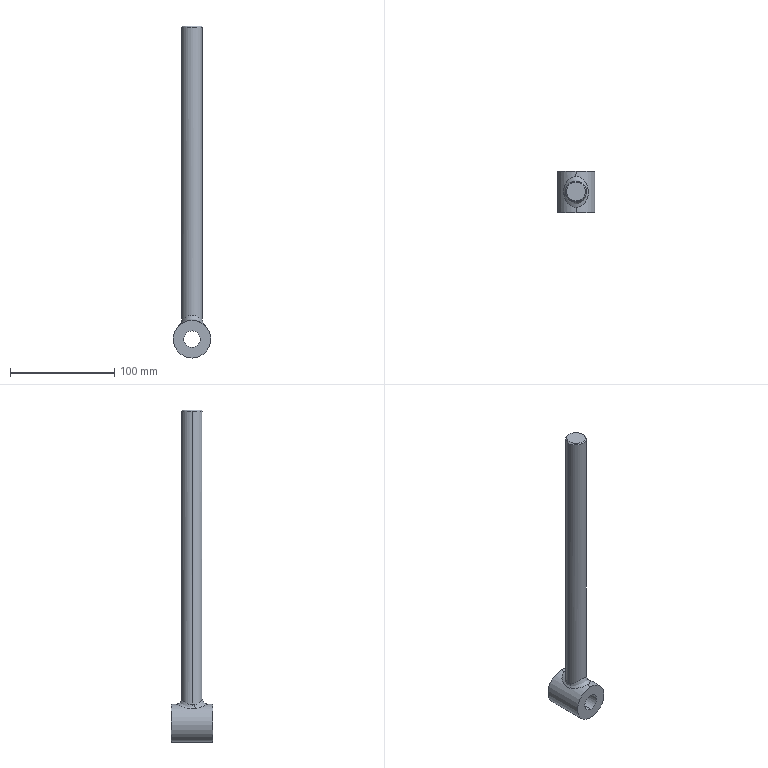Part | SolidWorks | 1 solid | 13 faces | box 36 x 40 x 318 mm | volume 121648 mm3 | cylinder 6 | plane 3 | cone 2 | spline 2 | commonest cylinder face diameters 16 x2 20 x2 36 x2
STEP:
#1=CARTESIAN_POINT('',(9.,0.,300.));
#2=VERTEX_POINT('',#1);
#3=CARTESIAN_POINT('',(-9.,0.,300.));
#4=VERTEX_POINT('',#3);
#5=CARTESIAN_POINT('',(0.,0.,300.));
#6=DIRECTION('',(0.,0.,1.));
#7=DIRECTION('',(1.,0.,0.));
#8=AXIS2_PLACEMENT_3D('',#5,#6,#7);
#9=CIRCLE('',#8,9.);
#10=EDGE_CURVE('',#2,#4,#9,.T.);
#11=ORIENTED_EDGE('',*,*,#10,.F.);
#12=CARTESIAN_POINT('',(10.,0.,299.));
#13=VERTEX_POINT('',#12);
#14=CARTESIAN_POINT('',(9.,0.,300.));
#15=DIRECTION('',(0.7071,0.,-0.7071));
#16=VECTOR('',#15,1000.);
#17=LINE('',#14,#16);
#18=EDGE_CURVE('',#2,#13,#17,.T.);
#19=ORIENTED_EDGE('',*,*,#18,.T.);
#20=CARTESIAN_POINT('',(-10.,0.,299.));
#21=VERTEX_POINT('',#20);
#22=CARTESIAN_POINT('',(0.,0.,299.));
#23=DIRECTION('',(0.,0.,-1.));
#24=DIRECTION('',(1.,0.,0.));
#25=AXIS2_PLACEMENT_3D('',#22,#23,#24);
#26=CIRCLE('',#25,10.);
#27=EDGE_CURVE('',#21,#13,#26,.T.);
#28=ORIENTED_EDGE('',*,*,#27,.F.);
#29=CARTESIAN_POINT('',(-9.,0.,300.));
#30=DIRECTION('',(-0.7071,0.,-0.7071));
#31=VECTOR('',#30,1000.);
#32=LINE('',#29,#31);
#33=EDGE_CURVE('',#4,#21,#32,.T.);
#34=ORIENTED_EDGE('',*,*,#33,.F.);
#35=EDGE_LOOP('',(#11,#19,#28,#34));
#36=FACE_OUTER_BOUND('',#35,.T.);
#37=CARTESIAN_POINT('',(0.,0.,300.));
#38=DIRECTION('',(0.,0.,-1.));
#39=DIRECTION('',(-1.,0.,0.));
#40=AXIS2_PLACEMENT_3D('',#37,#38,#39);
#41=CONICAL_SURFACE('',#40,9.,0.7854);
#42=ADVANCED_FACE('',(#36),#41,.T.);
#43=CARTESIAN_POINT('',(11.46,3.254,13.881));
#44=VERTEX_POINT('',#43);
#45=CARTESIAN_POINT('',(0.,-15.,18.));
#46=VERTEX_POINT('',#45);
#47=CARTESIAN_POINT('',(11.46,3.254,13.881));
#48=CARTESIAN_POINT('',(11.548,2.746,13.808));
#49=CARTESIAN_POINT('',(11.615,2.233,13.751));
#50=CARTESIAN_POINT('',(11.709,1.199,13.672));
#51=CARTESIAN_POINT('',(11.734,0.6762,13.649));
#52=CARTESIAN_POINT('',(11.747,-0.8792,13.638));
#53=CARTESIAN_POINT('',(11.672,-1.908,13.704));
#54=CARTESIAN_POINT('',(11.433,-3.441,13.903));
#55=CARTESIAN_POINT('',(11.333,-3.946,13.985));
#56=CARTESIAN_POINT('',(11.093,-4.936,14.176));
#57=CARTESIAN_POINT('',(10.953,-5.422,14.285));
#58=CARTESIAN_POINT('',(10.632,-6.379,14.526));
#59=CARTESIAN_POINT('',(10.451,-6.851,14.657));
#60=CARTESIAN_POINT('',(10.05,-7.77,14.935));
#61=CARTESIAN_POINT('',(9.83,-8.216,15.081));
#62=CARTESIAN_POINT('',(9.351,-9.083,15.383));
#63=CARTESIAN_POINT('',(9.092,-9.504,15.538));
#64=CARTESIAN_POINT('',(8.531,-10.319,15.853));
#65=CARTESIAN_POINT('',(8.227,-10.715,16.014));
#66=CARTESIAN_POINT('',(7.262,-11.838,16.486));
#67=CARTESIAN_POINT('',(6.545,-12.509,16.79));
#68=CARTESIAN_POINT('',(5.326,-13.38,17.199));
#69=CARTESIAN_POINT('',(4.892,-13.65,17.329));
#70=CARTESIAN_POINT('',(3.994,-14.119,17.557));
#71=CARTESIAN_POINT('',(3.529,-14.32,17.657));
#72=CARTESIAN_POINT('',(2.807,-14.568,17.781));
#73=CARTESIAN_POINT('',(2.562,-14.642,17.819));
#74=CARTESIAN_POINT('',(2.063,-14.77,17.883));
#75=CARTESIAN_POINT('',(1.808,-14.825,17.911));
#76=CARTESIAN_POINT('',(1.035,-14.956,17.978));
#77=CARTESIAN_POINT('',(0.518,-15.,18.));
#78=CARTESIAN_POINT('',(0.,-15.,18.));
#79=B_SPLINE_CURVE_WITH_KNOTS('',3,(#47,#48,#49,#50,#51,#52,#53,#54,#55,#56,#57,#58,#59,#60,#61,#62,#63,#64,#65,#66,#67,#68,#69,#70,#71,#72,#73,#74,#75,#76,#77,#78),.UNSPECIFIED.,.F.,.F.,(4,2,2,2,2,2,2,2,2,2,2,2,2,2,2,4),(0.04024,0.04181,0.04337,0.04651,0.04808,0.04964,0.05121,0.05278,0.05435,0.05592,0.05905,0.06062,0.06219,0.06297,0.06375,0.06532),.UNSPECIFIED.);
#80=EDGE_CURVE('',#44,#46,#79,.T.);
#81=ORIENTED_EDGE('',*,*,#80,.F.);
#82=CARTESIAN_POINT('',(9.762,2.169,17.737));
#83=VERTEX_POINT('',#82);
#84=CARTESIAN_POINT('',(14.643,3.254,17.737));
#85=DIRECTION('',(-0.2135,0.9609,0.1763));
#86=DIRECTION('',(-0.9762,-0.2169,0.));
#87=AXIS2_PLACEMENT_3D('',#84,#85,#86);
#88=CIRCLE('',#87,5.);
#89=EDGE_CURVE('',#44,#83,#88,.T.);
#90=ORIENTED_EDGE('',*,*,#89,.T.);
#91=CARTESIAN_POINT('',(10.,0.,17.436));
#92=VERTEX_POINT('',#91);
#93=CARTESIAN_POINT('',(10.,0.,17.436));
#94=CARTESIAN_POINT('',(10.,0.3703,17.436));
#95=CARTESIAN_POINT('',(9.979,0.7418,17.463));
#96=CARTESIAN_POINT('',(9.899,1.467,17.566));
#97=CARTESIAN_POINT('',(9.839,1.822,17.641));
#98=CARTESIAN_POINT('',(9.762,2.169,17.737));
#99=B_SPLINE_CURVE_WITH_KNOTS('',3,(#93,#94,#95,#96,#97,#98),.UNSPECIFIED.,.F.,.F.,(4,2,4),(0.03372,0.03482,0.03592),.UNSPECIFIED.);
#100=EDGE_CURVE('',#92,#83,#99,.T.);
#101=ORIENTED_EDGE('',*,*,#100,.F.);
#102=CARTESIAN_POINT('',(-9.771,-2.127,17.725));
#103=VERTEX_POINT('',#102);
#104=CARTESIAN_POINT('',(-9.771,-2.127,17.725));
#105=CARTESIAN_POINT('',(-9.634,-2.757,17.895));
#106=CARTESIAN_POINT('',(-9.445,-3.34,18.124));
#107=CARTESIAN_POINT('',(-9.096,-4.166,18.517));
#108=CARTESIAN_POINT('',(-8.968,-4.433,18.657));
#109=CARTESIAN_POINT('',(-8.692,-4.954,18.949));
#110=CARTESIAN_POINT('',(-8.542,-5.207,19.102));
#111=CARTESIAN_POINT('',(-8.066,-5.939,19.568));
#112=CARTESIAN_POINT('',(-7.714,-6.39,19.889));
#113=CARTESIAN_POINT('',(-6.931,-7.231,20.527));
#114=CARTESIAN_POINT('',(-6.499,-7.623,20.846));
#115=CARTESIAN_POINT('',(-5.565,-8.329,21.445));
#116=CARTESIAN_POINT('',(-5.064,-8.645,21.726));
#117=CARTESIAN_POINT('',(-4.247,-9.058,22.104));
#118=CARTESIAN_POINT('',(-3.964,-9.186,22.223));
#119=CARTESIAN_POINT('',(-3.386,-9.414,22.437));
#120=CARTESIAN_POINT('',(-3.09,-9.516,22.533));
#121=CARTESIAN_POINT('',(-2.483,-9.692,22.701));
#122=CARTESIAN_POINT('',(-2.172,-9.767,22.773));
#123=CARTESIAN_POINT('',(-1.532,-9.887,22.89));
#124=CARTESIAN_POINT('',(-1.205,-9.933,22.934));
#125=CARTESIAN_POINT('',(-0.5528,-9.99,22.99));
#126=CARTESIAN_POINT('',(-0.2258,-10.003,23.003));
#127=CARTESIAN_POINT('',(0.4303,-9.996,22.996));
#128=CARTESIAN_POINT('',(0.7605,-9.977,22.977));
#129=CARTESIAN_POINT('',(1.418,-9.905,22.907));
#130=CARTESIAN_POINT('',(1.743,-9.852,22.856));
#131=CARTESIAN_POINT('',(2.373,-9.72,22.728));
#132=CARTESIAN_POINT('',(2.68,-9.639,22.651));
#133=CARTESIAN_POINT('',(3.28,-9.452,22.472));
#134=CARTESIAN_POINT('',(3.572,-9.345,22.372));
#135=CARTESIAN_POINT('',(4.144,-9.106,22.149));
#136=CARTESIAN_POINT('',(4.423,-8.974,22.026));
#137=CARTESIAN_POINT('',(5.225,-8.548,21.64));
#138=CARTESIAN_POINT('',(5.716,-8.226,21.355));
#139=CARTESIAN_POINT('',(6.4,-7.689,20.904));
#140=CARTESIAN_POINT('',(6.619,-7.502,20.75));
#141=CARTESIAN_POINT('',(7.04,-7.108,20.435));
#142=CARTESIAN_POINT('',(7.243,-6.9,20.275));
#143=CARTESIAN_POINT('',(7.82,-6.259,19.795));
#144=CARTESIAN_POINT('',(8.166,-5.802,19.475));
#145=CARTESIAN_POINT('',(8.782,-4.818,18.862));
#146=CARTESIAN_POINT('',(9.055,-4.287,18.566));
#147=CARTESIAN_POINT('',(9.392,-3.448,18.182));
#148=CARTESIAN_POINT('',(9.493,-3.16,18.063));
#149=CARTESIAN_POINT('',(9.67,-2.566,17.85));
#150=CARTESIAN_POINT('',(9.747,-2.258,17.755));
#151=CARTESIAN_POINT('',(9.935,-1.311,17.521));
#152=CARTESIAN_POINT('',(10.,-0.6645,17.436));
#153=CARTESIAN_POINT('',(10.,0.,17.436));
#154=B_SPLINE_CURVE_WITH_KNOTS('',3,(#104,#105,#106,#107,#108,#109,#110,#111,#112,#113,#114,#115,#116,#117,#118,#119,#120,#121,#122,#123,#124,#125,#126,#127,#128,#129,#130,#131,#132,#133,#134,#135,#136,#137,#138,#139,#140,#141,#142,#143,#144,#145,#146,#147,#148,#149,#150,#151,#152,#153),.UNSPECIFIED.,.F.,.F.,(4,2,2,2,2,2,2,2,2,2,2,2,2,2,2,2,2,2,2,2,2,2,2,2,4),(0.002159,0.004132,0.005118,0.006104,0.008077,0.01005,0.01202,0.01301,0.01399,0.01498,0.01597,0.01695,0.01794,0.01893,0.01991,0.0209,0.02189,0.02386,0.02484,0.02583,0.0278,0.02978,0.03076,0.03175,0.03372),.UNSPECIFIED.);
#155=EDGE_CURVE('',#103,#92,#154,.T.);
#156=ORIENTED_EDGE('',*,*,#155,.F.);
#157=CARTESIAN_POINT('',(-11.47,-3.191,13.872));
#158=VERTEX_POINT('',#157);
#159=CARTESIAN_POINT('',(-14.657,-3.191,17.725));
#160=DIRECTION('',(0.2095,-0.9623,0.1733));
#161=DIRECTION('',(0.9771,0.2127,0.));
#162=AXIS2_PLACEMENT_3D('',#159,#160,#161);
#163=CIRCLE('',#162,5.);
#164=EDGE_CURVE('',#158,#103,#163,.T.);
#165=ORIENTED_EDGE('',*,*,#164,.F.);
#166=CARTESIAN_POINT('',(0.,-15.,18.));
#167=CARTESIAN_POINT('',(-0.3821,-15.,18.));
#168=CARTESIAN_POINT('',(-0.7649,-14.976,17.988));
#169=CARTESIAN_POINT('',(-1.532,-14.88,17.939));
#170=CARTESIAN_POINT('',(-1.914,-14.807,17.902));
#171=CARTESIAN_POINT('',(-3.024,-14.526,17.76));
#172=CARTESIAN_POINT('',(-3.723,-14.255,17.624));
#173=CARTESIAN_POINT('',(-4.721,-13.741,17.373));
#174=CARTESIAN_POINT('',(-5.047,-13.551,17.281));
#175=CARTESIAN_POINT('',(-5.669,-13.143,17.087));
#176=CARTESIAN_POINT('',(-5.967,-12.925,16.985));
#177=CARTESIAN_POINT('',(-6.825,-12.235,16.667));
#178=CARTESIAN_POINT('',(-7.35,-11.725,16.44));
#179=CARTESIAN_POINT('',(-8.318,-10.618,15.972));
#180=CARTESIAN_POINT('',(-8.75,-10.032,15.737));
#181=CARTESIAN_POINT('',(-9.527,-8.8,15.279));
#182=CARTESIAN_POINT('',(-9.872,-8.155,15.056));
#183=CARTESIAN_POINT('',(-10.48,-6.803,14.639));
#184=CARTESIAN_POINT('',(-10.739,-6.106,14.448));
#185=CARTESIAN_POINT('',(-11.17,-4.677,14.118));
#186=CARTESIAN_POINT('',(-11.342,-3.945,13.978));
#187=CARTESIAN_POINT('',(-11.47,-3.191,13.872));
#188=B_SPLINE_CURVE_WITH_KNOTS('',3,(#166,#167,#168,#169,#170,#171,#172,#173,#174,#175,#176,#177,#178,#179,#180,#181,#182,#183,#184,#185,#186,#187),.UNSPECIFIED.,.F.,.F.,(4,2,2,2,2,2,2,2,2,2,4),(0.06532,0.06648,0.06763,0.06995,0.0711,0.07226,0.07457,0.07688,0.0792,0.08151,0.08382),.UNSPECIFIED.);
#189=EDGE_CURVE('',#46,#158,#188,.T.);
#190=ORIENTED_EDGE('',*,*,#189,.F.);
#191=EDGE_LOOP('',(#81,#90,#101,#156,#165,#190));
#192=FACE_OUTER_BOUND('',#191,.T.);
#193=CARTESIAN_POINT('',(11.46,3.254,13.881));
#194=CARTESIAN_POINT('',(9.669,2.585,15.359));
#195=CARTESIAN_POINT('',(9.762,2.169,17.737));
#196=CARTESIAN_POINT('',(11.545,2.763,13.81));
#197=CARTESIAN_POINT('',(9.77,2.2,15.294));
#198=CARTESIAN_POINT('',(9.835,1.842,17.647));
#199=CARTESIAN_POINT('',(11.611,2.265,13.754));
#200=CARTESIAN_POINT('',(9.848,1.805,15.243));
#201=CARTESIAN_POINT('',(9.891,1.51,17.575));
#202=CARTESIAN_POINT('',(11.705,1.255,13.675));
#203=CARTESIAN_POINT('',(9.959,1.003,15.169));
#204=CARTESIAN_POINT('',(9.971,0.837,17.474));
#205=CARTESIAN_POINT('',(11.731,0.7419,13.652));
#206=CARTESIAN_POINT('',(9.991,0.5923,15.148));
#207=CARTESIAN_POINT('',(9.993,0.4946,17.444));
#208=CARTESIAN_POINT('',(11.75,-0.7804,13.636));
#209=CARTESIAN_POINT('',(10.013,-0.6225,15.133));
#210=CARTESIAN_POINT('',(10.009,-0.5202,17.424));
#211=CARTESIAN_POINT('',(11.683,-1.783,13.695));
#212=CARTESIAN_POINT('',(9.932,-1.428,15.189));
#213=CARTESIAN_POINT('',(9.952,-1.189,17.499));
#214=CARTESIAN_POINT('',(11.5,-3.022,13.847));
#215=CARTESIAN_POINT('',(9.717,-2.403,15.328));
#216=CARTESIAN_POINT('',(9.796,-2.015,17.694));
#217=CARTESIAN_POINT('',(11.459,-3.27,13.882));
#218=CARTESIAN_POINT('',(9.668,-2.598,15.36));
#219=CARTESIAN_POINT('',(9.761,-2.18,17.738));
#220=CARTESIAN_POINT('',(11.367,-3.757,13.957));
#221=CARTESIAN_POINT('',(9.56,-2.98,15.428));
#222=CARTESIAN_POINT('',(9.683,-2.505,17.834));
#223=CARTESIAN_POINT('',(11.316,-3.997,13.998));
#224=CARTESIAN_POINT('',(9.501,-3.168,15.466));
#225=CARTESIAN_POINT('',(9.64,-2.665,17.886));
#226=CARTESIAN_POINT('',(11.152,-4.71,14.13));
#227=CARTESIAN_POINT('',(9.309,-3.724,15.584));
#228=CARTESIAN_POINT('',(9.5,-3.14,18.055));
#229=CARTESIAN_POINT('',(11.026,-5.173,14.229));
#230=CARTESIAN_POINT('',(9.162,-4.081,15.673));
#231=CARTESIAN_POINT('',(9.392,-3.448,18.182));
#232=CARTESIAN_POINT('',(10.596,-6.529,14.555));
#233=CARTESIAN_POINT('',(8.665,-5.118,15.961));
#234=CARTESIAN_POINT('',(9.027,-4.352,18.598));
#235=CARTESIAN_POINT('',(10.241,-7.394,14.811));
#236=CARTESIAN_POINT('',(8.259,-5.759,16.18));
#237=CARTESIAN_POINT('',(8.724,-4.93,18.925));
#238=CARTESIAN_POINT('',(9.424,-8.995,15.344));
#239=CARTESIAN_POINT('',(7.362,-6.897,16.609));
#240=CARTESIAN_POINT('',(8.028,-5.997,19.606));
#241=CARTESIAN_POINT('',(8.961,-9.738,15.622));
#242=CARTESIAN_POINT('',(6.864,-7.398,16.822));
#243=CARTESIAN_POINT('',(7.633,-6.492,19.962));
#244=CARTESIAN_POINT('',(7.917,-11.117,16.176));
#245=CARTESIAN_POINT('',(5.802,-8.271,17.209));
#246=CARTESIAN_POINT('',(6.744,-7.411,20.67));
#247=CARTESIAN_POINT('',(7.349,-11.736,16.445));
#248=CARTESIAN_POINT('',(5.25,-8.629,17.377));
#249=CARTESIAN_POINT('',(6.26,-7.824,21.013));
#250=CARTESIAN_POINT('',(6.429,-12.56,16.816));
#251=CARTESIAN_POINT('',(4.425,-9.06,17.581));
#252=CARTESIAN_POINT('',(5.477,-8.373,21.487));
#253=CARTESIAN_POINT('',(6.111,-12.817,16.935));
#254=CARTESIAN_POINT('',(4.148,-9.187,17.641));
#255=CARTESIAN_POINT('',(5.205,-8.545,21.639));
#256=CARTESIAN_POINT('',(5.449,-13.295,17.159));
#257=CARTESIAN_POINT('',(3.594,-9.411,17.746));
#258=CARTESIAN_POINT('',(4.642,-8.863,21.925));
#259=CARTESIAN_POINT('',(5.103,-13.518,17.265));
#260=CARTESIAN_POINT('',(3.317,-9.506,17.791));
#261=CARTESIAN_POINT('',(4.347,-9.012,22.061));
#262=CARTESIAN_POINT('',(4.04,-14.119,17.556));
#263=CARTESIAN_POINT('',(2.498,-9.75,17.902));
#264=CARTESIAN_POINT('',(3.441,-9.412,22.433));
#265=CARTESIAN_POINT('',(3.302,-14.429,17.711));
#266=CARTESIAN_POINT('',(1.991,-9.847,17.943));
#267=CARTESIAN_POINT('',(2.813,-9.62,22.631));
#268=CARTESIAN_POINT('',(2.342,-14.701,17.848));
#269=CARTESIAN_POINT('',(1.385,-9.924,17.973));
#270=CARTESIAN_POINT('',(1.995,-9.8,22.806));
#271=CARTESIAN_POINT('',(2.148,-14.749,17.872));
#272=CARTESIAN_POINT('',(1.265,-9.937,17.978));
#273=CARTESIAN_POINT('',(1.83,-9.833,22.837));
#274=CARTESIAN_POINT('',(1.756,-14.833,17.915));
#275=CARTESIAN_POINT('',(1.025,-9.959,17.986));
#276=CARTESIAN_POINT('',(1.496,-9.889,22.892));
#277=CARTESIAN_POINT('',(1.558,-14.869,17.934));
#278=CARTESIAN_POINT('',(0.9062,-9.968,17.989));
#279=CARTESIAN_POINT('',(1.327,-9.913,22.915));
#280=CARTESIAN_POINT('',(0.9645,-14.958,17.979));
#281=CARTESIAN_POINT('',(0.5542,-9.99,17.997));
#282=CARTESIAN_POINT('',(0.8216,-9.972,22.973));
#283=CARTESIAN_POINT('',(0.5691,-14.991,17.995));
#284=CARTESIAN_POINT('',(0.3268,-9.998,17.999));
#285=CARTESIAN_POINT('',(0.4848,-9.994,22.994));
#286=CARTESIAN_POINT('',(-0.2213,-15.006,18.003));
#287=CARTESIAN_POINT('',(-0.1272,-10.001,18.));
#288=CARTESIAN_POINT('',(-0.1885,-10.004,23.004));
#289=CARTESIAN_POINT('',(-0.6162,-14.988,17.994));
#290=CARTESIAN_POINT('',(-0.3527,-9.997,17.999));
#291=CARTESIAN_POINT('',(-0.5249,-9.992,22.992));
#292=CARTESIAN_POINT('',(-1.406,-14.901,17.949));
#293=CARTESIAN_POINT('',(-0.8139,-9.976,17.992));
#294=CARTESIAN_POINT('',(-1.197,-9.934,22.935));
#295=CARTESIAN_POINT('',(-1.803,-14.831,17.914));
#296=CARTESIAN_POINT('',(-1.05,-9.959,17.986));
#297=CARTESIAN_POINT('',(-1.536,-9.887,22.89));
#298=CARTESIAN_POINT('',(-2.972,-14.547,17.77));
#299=CARTESIAN_POINT('',(-1.773,-9.882,17.957));
#300=CARTESIAN_POINT('',(-2.532,-9.698,22.707));
#301=CARTESIAN_POINT('',(-3.719,-14.262,17.627));
#302=CARTESIAN_POINT('',(-2.272,-9.798,17.923));
#303=CARTESIAN_POINT('',(-3.168,-9.508,22.524));
#304=CARTESIAN_POINT('',(-4.796,-13.7,17.353));
#305=CARTESIAN_POINT('',(-3.078,-9.581,17.825));
#306=CARTESIAN_POINT('',(-4.085,-9.133,22.174));
#307=CARTESIAN_POINT('',(-5.149,-13.489,17.252));
#308=CARTESIAN_POINT('',(-3.354,-9.495,17.785));
#309=CARTESIAN_POINT('',(-4.386,-8.993,22.044));
#310=CARTESIAN_POINT('',(-5.827,-13.031,17.035));
#311=CARTESIAN_POINT('',(-3.906,-9.29,17.689));
#312=CARTESIAN_POINT('',(-4.964,-8.687,21.766));
#313=CARTESIAN_POINT('',(-6.153,-12.783,16.919));
#314=CARTESIAN_POINT('',(-4.185,-9.171,17.634));
#315=CARTESIAN_POINT('',(-5.242,-8.522,21.619));
#316=CARTESIAN_POINT('',(-6.784,-12.251,16.676));
#317=CARTESIAN_POINT('',(-4.742,-8.9,17.505));
#318=CARTESIAN_POINT('',(-5.779,-8.168,21.308));
#319=CARTESIAN_POINT('',(-7.087,-11.967,16.549));
#320=CARTESIAN_POINT('',(-5.021,-8.747,17.433));
#321=CARTESIAN_POINT('',(-6.037,-7.978,21.146));
#322=CARTESIAN_POINT('',(-7.672,-11.363,16.286));
#323=CARTESIAN_POINT('',(-5.576,-8.403,17.273));
#324=CARTESIAN_POINT('',(-6.536,-7.575,20.81));
#325=CARTESIAN_POINT('',(-7.955,-11.041,16.15));
#326=CARTESIAN_POINT('',(-5.852,-8.212,17.185));
#327=CARTESIAN_POINT('',(-6.776,-7.361,20.636));
#328=CARTESIAN_POINT('',(-8.755,-10.038,15.739));
#329=CARTESIAN_POINT('',(-6.649,-7.594,16.907));
#330=CARTESIAN_POINT('',(-7.458,-6.692,20.11));
#331=CARTESIAN_POINT('',(-9.233,-9.313,15.46));
#332=CARTESIAN_POINT('',(-7.157,-7.114,16.699));
#333=CARTESIAN_POINT('',(-7.865,-6.209,19.754));
#334=CARTESIAN_POINT('',(-9.869,-8.136,15.055));
#335=CARTESIAN_POINT('',(-7.854,-6.283,16.376));
#336=CARTESIAN_POINT('',(-8.407,-5.424,19.237));
#337=CARTESIAN_POINT('',(-10.068,-7.728,14.922));
#338=CARTESIAN_POINT('',(-8.075,-5.99,16.267));
#339=CARTESIAN_POINT('',(-8.577,-5.152,19.068));
#340=CARTESIAN_POINT('',(-10.438,-6.881,14.666));
#341=CARTESIAN_POINT('',(-8.489,-5.371,16.053));
#342=CARTESIAN_POINT('',(-8.892,-4.587,18.74));
#343=CARTESIAN_POINT('',(-10.606,-6.447,14.545));
#344=CARTESIAN_POINT('',(-8.68,-5.047,15.949));
#345=CARTESIAN_POINT('',(-9.035,-4.298,18.585));
#346=CARTESIAN_POINT('',(-11.062,-5.113,14.205));
#347=CARTESIAN_POINT('',(-9.2,-4.044,15.655));
#348=CARTESIAN_POINT('',(-9.423,-3.408,18.15));
#349=CARTESIAN_POINT('',(-11.302,-4.179,14.011));
#350=CARTESIAN_POINT('',(-9.483,-3.318,15.479));
#351=CARTESIAN_POINT('',(-9.628,-2.786,17.903));
#352=CARTESIAN_POINT('',(-11.47,-3.191,13.872));
#353=CARTESIAN_POINT('',(-9.682,-2.536,15.351));
#354=CARTESIAN_POINT('',(-9.771,-2.127,17.725));
#355=(BOUNDED_SURFACE()B_SPLINE_SURFACE(3,2,((#193,#194,#195),(#196,#197,#198),(#199,#200,#201),(#202,#203,#204),(#205,#206,#207),(#208,#209,#210),(#211,#212,#213),(#214,#215,#216),(#217,#218,#219),(#220,#221,#222),(#223,#224,#225),(#226,#227,#228),(#229,#230,#231),(#232,#233,#234),(#235,#236,#237),(#238,#239,#240),(#241,#242,#243),(#244,#245,#246),(#247,#248,#249),(#250,#251,#252),(#253,#254,#255),(#256,#257,#258),(#259,#260,#261),(#262,#263,#264),(#265,#266,#267),(#268,#269,#270),(#271,#272,#273),(#274,#275,#276),(#277,#278,#279),(#280,#281,#282),(#283,#284,#285),(#286,#287,#288),(#289,#290,#291),(#292,#293,#294),(#295,#296,#297),(#298,#299,#300),(#301,#302,#303),(#304,#305,#306),(#307,#308,#309),(#310,#311,#312),(#313,#314,#315),(#316,#317,#318),(#319,#320,#321),(#322,#323,#324),(#325,#326,#327),(#328,#329,#330),(#331,#332,#333),(#334,#335,#336),(#337,#338,#339),(#340,#341,#342),(#343,#344,#345),(#346,#347,#348),(#349,#350,#351),(#352,#353,#354)),.UNSPECIFIED.,.F.,.F.,.F.)B_SPLINE_SURFACE_WITH_KNOTS((4,2,2,2,2,2,2,2,2,2,2,2,2,2,2,2,2,2,2,2,2,2,2,2,2,2,4),(3,3),(0.04847,0.04999,0.0515,0.05453,0.05529,0.05605,0.05756,0.06059,0.06362,0.06665,0.06816,0.06968,0.07271,0.07346,0.07422,0.07574,0.07725,0.07877,0.0818,0.08331,0.08482,0.08634,0.08785,0.09088,0.0924,0.09391,0.09694),(0.,1.),.UNSPECIFIED.)GEOMETRIC_REPRESENTATION_ITEM()RATIONAL_B_SPLINE_SURFACE(((1.,0.9004,1.),(1.,0.903,1.),(1.,0.905,1.),(1.,0.9078,1.),(1.,0.9087,1.),(1.,0.9092,1.),(1.,0.9072,1.),(1.,0.9016,1.),(1.,0.9004,1.),(1.,0.8976,1.),(1.,0.8961,1.),(1.,0.8912,1.),(1.,0.8875,1.),(1.,0.875,1.),(1.,0.8648,1.),(1.,0.8425,1.),(1.,0.8304,1.),(1.,0.8049,1.),(1.,0.7919,1.),(1.,0.7731,1.),(1.,0.7669,1.),(1.,0.755,1.),(1.,0.7492,1.),(1.,0.7332,1.),(1.,0.7242,1.),(1.,0.7162,1.),(1.,0.7147,1.),(1.,0.7122,1.),(1.,0.7111,1.),(1.,0.7084,1.),(1.,0.7074,1.),(1.,0.7069,1.),(1.,0.7075,1.),(1.,0.7101,1.),(1.,0.7123,1.),(1.,0.7208,1.),(1.,0.7291,1.),(1.,0.7444,1.),(1.,0.75,1.),(1.,0.7616,1.),(1.,0.7677,1.),(1.,0.7802,1.),(1.,0.7866,1.),(1.,0.7995,1.),(1.,0.806,1.),(1.,0.8252,1.),(1.,0.8375,1.),(1.,0.8546,1.),(1.,0.8601,1.),(1.,0.8705,1.),(1.,0.8753,1.),(1.,0.8885,1.),(1.,0.8957,1.),(1.,0.9007,1.)))REPRESENTATION_ITEM('')SURFACE());
#356=ADVANCED_FACE('',(#192),#355,.F.);
#357=ORIENTED_EDGE('',*,*,#27,.T.);
#358=CARTESIAN_POINT('',(10.,0.,300.));
#359=DIRECTION('',(0.,0.,-1.));
#360=VECTOR('',#359,1000.);
#361=LINE('',#358,#360);
#362=EDGE_CURVE('',#13,#92,#361,.T.);
#363=ORIENTED_EDGE('',*,*,#362,.T.);
#364=ORIENTED_EDGE('',*,*,#100,.T.);
#365=CARTESIAN_POINT('',(-10.,0.,17.436));
#366=VERTEX_POINT('',#365);
#367=CARTESIAN_POINT('',(9.762,2.169,17.737));
#368=CARTESIAN_POINT('',(9.692,2.482,17.823));
#369=CARTESIAN_POINT('',(9.608,2.788,17.925));
#370=CARTESIAN_POINT('',(9.419,3.374,18.15));
#371=CARTESIAN_POINT('',(9.312,3.656,18.274));
#372=CARTESIAN_POINT('',(8.961,4.477,18.668));
#373=CARTESIAN_POINT('',(8.686,4.99,18.963));
#374=CARTESIAN_POINT('',(8.209,5.718,19.428));
#375=CARTESIAN_POINT('',(8.039,5.954,19.588));
#376=CARTESIAN_POINT('',(7.684,6.406,19.906));
#377=CARTESIAN_POINT('',(7.498,6.623,20.066));
#378=CARTESIAN_POINT('',(6.911,7.25,20.542));
#379=CARTESIAN_POINT('',(6.484,7.636,20.857));
#380=CARTESIAN_POINT('',(5.542,8.344,21.459));
#381=CARTESIAN_POINT('',(5.039,8.659,21.739));
#382=CARTESIAN_POINT('',(4.227,9.068,22.113));
#383=CARTESIAN_POINT('',(3.947,9.193,22.229));
#384=CARTESIAN_POINT('',(3.365,9.422,22.444));
#385=CARTESIAN_POINT('',(3.065,9.524,22.54));
#386=CARTESIAN_POINT('',(2.153,9.786,22.791));
#387=CARTESIAN_POINT('',(1.522,9.906,22.908));
#388=CARTESIAN_POINT('',(0.5349,9.991,22.991));
#389=CARTESIAN_POINT('',(0.2044,10.003,23.003));
#390=CARTESIAN_POINT('',(-0.451,9.995,22.995));
#391=CARTESIAN_POINT('',(-0.7772,9.975,22.976));
#392=CARTESIAN_POINT('',(-1.752,9.867,22.87));
#393=CARTESIAN_POINT('',(-2.4,9.728,22.735));
#394=CARTESIAN_POINT('',(-3.604,9.349,22.375));
#395=CARTESIAN_POINT('',(-4.165,9.111,22.151));
#396=CARTESIAN_POINT('',(-4.959,8.689,21.768));
#397=CARTESIAN_POINT('',(-5.215,8.538,21.632));
#398=CARTESIAN_POINT('',(-5.713,8.213,21.348));
#399=CARTESIAN_POINT('',(-5.954,8.04,21.199));
#400=CARTESIAN_POINT('',(-6.641,7.499,20.744));
#401=CARTESIAN_POINT('',(-7.059,7.107,20.429));
#402=CARTESIAN_POINT('',(-7.823,6.255,19.792));
#403=CARTESIAN_POINT('',(-8.172,5.792,19.469));
#404=CARTESIAN_POINT('',(-8.787,4.809,18.857));
#405=CARTESIAN_POINT('',(-9.054,4.289,18.567));
#406=CARTESIAN_POINT('',(-9.391,3.45,18.183));
#407=CARTESIAN_POINT('',(-9.493,3.158,18.063));
#408=CARTESIAN_POINT('',(-9.672,2.559,17.848));
#409=CARTESIAN_POINT('',(-9.748,2.254,17.754));
#410=CARTESIAN_POINT('',(-9.871,1.632,17.601));
#411=CARTESIAN_POINT('',(-9.919,1.315,17.54));
#412=CARTESIAN_POINT('',(-9.983,0.666,17.457));
#413=CARTESIAN_POINT('',(-10.,0.3343,17.436));
#414=CARTESIAN_POINT('',(-10.,0.,17.436));
#415=B_SPLINE_CURVE_WITH_KNOTS('',3,(#367,#368,#369,#370,#371,#372,#373,#374,#375,#376,#377,#378,#379,#380,#381,#382,#383,#384,#385,#386,#387,#388,#389,#390,#391,#392,#393,#394,#395,#396,#397,#398,#399,#400,#401,#402,#403,#404,#405,#406,#407,#408,#409,#410,#411,#412,#413,#414),.UNSPECIFIED.,.F.,.F.,(4,2,2,2,2,2,2,2,2,2,2,2,2,2,2,2,2,2,2,2,2,2,2,4),(0.03592,0.03691,0.0379,0.03987,0.04086,0.04185,0.04382,0.0458,0.04679,0.04778,0.04975,0.05074,0.05173,0.05371,0.05568,0.05667,0.05766,0.05964,0.06161,0.06359,0.06458,0.06556,0.06655,0.06754),.UNSPECIFIED.);
#416=EDGE_CURVE('',#83,#366,#415,.T.);
#417=ORIENTED_EDGE('',*,*,#416,.T.);
#418=CARTESIAN_POINT('',(-10.,0.,300.));
#419=DIRECTION('',(0.,0.,-1.));
#420=VECTOR('',#419,1000.);
#421=LINE('',#418,#420);
#422=EDGE_CURVE('',#21,#366,#421,.T.);
#423=ORIENTED_EDGE('',*,*,#422,.F.);
#424=EDGE_LOOP('',(#357,#363,#364,#417,#423));
#425=FACE_OUTER_BOUND('',#424,.T.);
#426=CARTESIAN_POINT('',(0.,0.,300.));
#427=DIRECTION('',(0.,0.,-1.));
#428=DIRECTION('',(-1.,0.,0.));
#429=AXIS2_PLACEMENT_3D('',#426,#427,#428);
#430=CYLINDRICAL_SURFACE('',#429,10.);
#431=ADVANCED_FACE('',(#425),#430,.T.);
#432=CARTESIAN_POINT('',(0.,20.,-8.));
#433=VERTEX_POINT('',#432);
#434=CARTESIAN_POINT('',(0.,20.,8.));
#435=VERTEX_POINT('',#434);
#436=CARTESIAN_POINT('',(0.,20.,0.));
#437=DIRECTION('',(0.,1.,0.));
#438=DIRECTION('',(0.,0.,1.));
#439=AXIS2_PLACEMENT_3D('',#436,#437,#438);
#440=CIRCLE('',#439,8.);
#441=EDGE_CURVE('',#433,#435,#440,.T.);
#442=ORIENTED_EDGE('',*,*,#441,.T.);
#443=CARTESIAN_POINT('',(0.,-20.,8.));
#444=VERTEX_POINT('',#443);
#445=CARTESIAN_POINT('',(0.,20.,8.));
#446=DIRECTION('',(0.,-1.,0.));
#447=VECTOR('',#446,1000.);
#448=LINE('',#445,#447);
#449=EDGE_CURVE('',#435,#444,#448,.T.);
#450=ORIENTED_EDGE('',*,*,#449,.T.);
#451=CARTESIAN_POINT('',(0.,-20.,-8.));
#452=VERTEX_POINT('',#451);
#453=CARTESIAN_POINT('',(0.,-20.,0.));
#454=DIRECTION('',(0.,1.,0.));
#455=DIRECTION('',(0.,0.,1.));
#456=AXIS2_PLACEMENT_3D('',#453,#454,#455);
#457=CIRCLE('',#456,8.);
#458=EDGE_CURVE('',#452,#444,#457,.T.);
#459=ORIENTED_EDGE('',*,*,#458,.F.);
#460=CARTESIAN_POINT('',(0.,20.,-8.));
#461=DIRECTION('',(0.,-1.,0.));
#462=VECTOR('',#461,1000.);
#463=LINE('',#460,#462);
#464=EDGE_CURVE('',#433,#452,#463,.T.);
#465=ORIENTED_EDGE('',*,*,#464,.F.);
#466=EDGE_LOOP('',(#442,#450,#459,#465));
#467=FACE_OUTER_BOUND('',#466,.T.);
#468=CARTESIAN_POINT('',(0.,20.,0.));
#469=DIRECTION('',(0.,-1.,0.));
#470=DIRECTION('',(0.,0.,-1.));
#471=AXIS2_PLACEMENT_3D('',#468,#469,#470);
#472=CYLINDRICAL_SURFACE('',#471,8.);
#473=ADVANCED_FACE('',(#467),#472,.F.);
#474=CARTESIAN_POINT('',(0.,20.,18.));
#475=VERTEX_POINT('',#474);
#476=CARTESIAN_POINT('',(0.,20.,-18.));
#477=VERTEX_POINT('',#476);
#478=CARTESIAN_POINT('',(0.,20.,0.));
#479=DIRECTION('',(0.,1.,0.));
#480=DIRECTION('',(1.,0.,0.));
#481=AXIS2_PLACEMENT_3D('',#478,#479,#480);
#482=CIRCLE('',#481,18.);
#483=EDGE_CURVE('',#475,#477,#482,.T.);
#484=ORIENTED_EDGE('',*,*,#483,.F.);
#485=CARTESIAN_POINT('',(0.,15.,18.));
#486=VERTEX_POINT('',#485);
#487=CARTESIAN_POINT('',(0.,20.,18.));
#488=DIRECTION('',(0.,-1.,0.));
#489=VECTOR('',#488,1000.);
#490=LINE('',#487,#489);
#491=EDGE_CURVE('',#475,#486,#490,.T.);
#492=ORIENTED_EDGE('',*,*,#491,.T.);
#493=CARTESIAN_POINT('',(0.,15.,18.));
#494=CARTESIAN_POINT('',(0.385,15.,18.));
#495=CARTESIAN_POINT('',(0.7744,14.975,17.987));
#496=CARTESIAN_POINT('',(1.536,14.879,17.938));
#497=CARTESIAN_POINT('',(1.909,14.808,17.902));
#498=CARTESIAN_POINT('',(2.64,14.624,17.809));
#499=CARTESIAN_POINT('',(2.998,14.51,17.752));
#500=CARTESIAN_POINT('',(3.7,14.243,17.619));
#501=CARTESIAN_POINT('',(4.045,14.089,17.543));
#502=CARTESIAN_POINT('',(5.047,13.574,17.292));
#503=CARTESIAN_POINT('',(5.661,13.169,17.097));
#504=CARTESIAN_POINT('',(6.806,12.252,16.675));
#505=CARTESIAN_POINT('',(7.338,11.737,16.445));
#506=CARTESIAN_POINT('',(8.297,10.644,15.983));
#507=CARTESIAN_POINT('',(8.728,10.062,15.749));
#508=CARTESIAN_POINT('',(9.509,8.831,15.29));
#509=CARTESIAN_POINT('',(9.858,8.18,15.065));
#510=CARTESIAN_POINT('',(10.463,6.844,14.651));
#511=CARTESIAN_POINT('',(10.721,6.156,14.461));
#512=CARTESIAN_POINT('',(11.046,5.092,14.213));
#513=CARTESIAN_POINT('',(11.144,4.732,14.136));
#514=CARTESIAN_POINT('',(11.318,4.001,13.997));
#515=CARTESIAN_POINT('',(11.394,3.629,13.935));
#516=CARTESIAN_POINT('',(11.46,3.254,13.881));
#517=B_SPLINE_CURVE_WITH_KNOTS('',3,(#493,#494,#495,#496,#497,#498,#499,#500,#501,#502,#503,#504,#505,#506,#507,#508,#509,#510,#511,#512,#513,#514,#515,#516),.UNSPECIFIED.,.F.,.F.,(4,2,2,2,2,2,2,2,2,2,2,4),(0.02175,0.02291,0.02406,0.02522,0.02637,0.02869,0.031,0.03331,0.03562,0.03793,0.03908,0.04024),.UNSPECIFIED.);
#518=EDGE_CURVE('',#486,#44,#517,.T.);
#519=ORIENTED_EDGE('',*,*,#518,.T.);
#520=ORIENTED_EDGE('',*,*,#80,.T.);
#521=CARTESIAN_POINT('',(0.,-20.,18.));
#522=VERTEX_POINT('',#521);
#523=CARTESIAN_POINT('',(0.,20.,18.));
#524=DIRECTION('',(0.,-1.,0.));
#525=VECTOR('',#524,1000.);
#526=LINE('',#523,#525);
#527=EDGE_CURVE('',#46,#522,#526,.T.);
#528=ORIENTED_EDGE('',*,*,#527,.T.);
#529=CARTESIAN_POINT('',(0.,-20.,-18.));
#530=VERTEX_POINT('',#529);
#531=CARTESIAN_POINT('',(0.,-20.,0.));
#532=DIRECTION('',(0.,1.,0.));
#533=DIRECTION('',(1.,0.,0.));
#534=AXIS2_PLACEMENT_3D('',#531,#532,#533);
#535=CIRCLE('',#534,18.);
#536=EDGE_CURVE('',#522,#530,#535,.T.);
#537=ORIENTED_EDGE('',*,*,#536,.T.);
#538=CARTESIAN_POINT('',(0.,20.,-18.));
#539=DIRECTION('',(0.,-1.,0.));
#540=VECTOR('',#539,1000.);
#541=LINE('',#538,#540);
#542=EDGE_CURVE('',#477,#530,#541,.T.);
#543=ORIENTED_EDGE('',*,*,#542,.F.);
#544=EDGE_LOOP('',(#484,#492,#519,#520,#528,#537,#543));
#545=FACE_OUTER_BOUND('',#544,.T.);
#546=CARTESIAN_POINT('',(0.,20.,0.));
#547=DIRECTION('',(0.,-1.,0.));
#548=DIRECTION('',(0.,0.,-1.));
#549=AXIS2_PLACEMENT_3D('',#546,#547,#548);
#550=CYLINDRICAL_SURFACE('',#549,18.);
#551=ADVANCED_FACE('',(#545),#550,.T.);
#552=ORIENTED_EDGE('',*,*,#491,.F.);
#553=CARTESIAN_POINT('',(0.,20.,0.));
#554=DIRECTION('',(0.,1.,0.));
#555=DIRECTION('',(1.,0.,0.));
#556=AXIS2_PLACEMENT_3D('',#553,#554,#555);
#557=CIRCLE('',#556,18.);
#558=EDGE_CURVE('',#477,#475,#557,.T.);
#559=ORIENTED_EDGE('',*,*,#558,.F.);
#560=ORIENTED_EDGE('',*,*,#542,.T.);
#561=CARTESIAN_POINT('',(0.,-20.,0.));
#562=DIRECTION('',(0.,1.,0.));
#563=DIRECTION('',(1.,0.,0.));
#564=AXIS2_PLACEMENT_3D('',#561,#562,#563);
#565=CIRCLE('',#564,18.);
#566=EDGE_CURVE('',#530,#522,#565,.T.);
#567=ORIENTED_EDGE('',*,*,#566,.T.);
#568=ORIENTED_EDGE('',*,*,#527,.F.);
#569=ORIENTED_EDGE('',*,*,#189,.T.);
#570=CARTESIAN_POINT('',(-11.47,-3.191,13.872));
#571=CARTESIAN_POINT('',(-11.644,-2.174,13.729));
#572=CARTESIAN_POINT('',(-11.733,-1.145,13.65));
#573=CARTESIAN_POINT('',(-11.742,0.4172,13.643));
#574=CARTESIAN_POINT('',(-11.723,0.9383,13.659));
#575=CARTESIAN_POINT('',(-11.645,1.969,13.726));
#576=CARTESIAN_POINT('',(-11.585,2.479,13.777));
#577=CARTESIAN_POINT('',(-11.344,3.996,13.977));
#578=CARTESIAN_POINT('',(-11.099,4.994,14.177));
#579=CARTESIAN_POINT('',(-10.457,6.894,14.656));
#580=CARTESIAN_POINT('',(-10.06,7.803,14.937));
#581=CARTESIAN_POINT('',(-9.338,9.106,15.391));
#582=CARTESIAN_POINT('',(-9.077,9.527,15.547));
#583=CARTESIAN_POINT('',(-8.518,10.335,15.86));
#584=CARTESIAN_POINT('',(-8.22,10.724,16.018));
#585=CARTESIAN_POINT('',(-7.579,11.468,16.33));
#586=CARTESIAN_POINT('',(-7.238,11.823,16.485));
#587=CARTESIAN_POINT('',(-6.506,12.499,16.788));
#588=CARTESIAN_POINT('',(-6.12,12.814,16.933));
#589=CARTESIAN_POINT('',(-5.31,13.391,17.204));
#590=CARTESIAN_POINT('',(-4.884,13.654,17.331));
#591=CARTESIAN_POINT('',(-3.987,14.122,17.559));
#592=CARTESIAN_POINT('',(-3.515,14.326,17.66));
#593=CARTESIAN_POINT('',(-2.539,14.659,17.827));
#594=CARTESIAN_POINT('',(-2.041,14.786,17.891));
#595=CARTESIAN_POINT('',(-1.032,14.956,17.978));
#596=CARTESIAN_POINT('',(-0.5203,15.,18.));
#597=CARTESIAN_POINT('',(0.,15.,18.));
#598=B_SPLINE_CURVE_WITH_KNOTS('',3,(#570,#571,#572,#573,#574,#575,#576,#577,#578,#579,#580,#581,#582,#583,#584,#585,#586,#587,#588,#589,#590,#591,#592,#593,#594,#595,#596,#597),.UNSPECIFIED.,.F.,.F.,(4,2,2,2,2,2,2,2,2,2,2,2,2,4),(0.08382,0.08694,0.0885,0.09007,0.09319,0.09631,0.09787,0.09943,0.101,0.1026,0.1041,0.1057,0.1072,0.1088),.UNSPECIFIED.);
#599=EDGE_CURVE('',#158,#486,#598,.T.);
#600=ORIENTED_EDGE('',*,*,#599,.T.);
#601=EDGE_LOOP('',(#552,#559,#560,#567,#568,#569,#600));
#602=FACE_OUTER_BOUND('',#601,.T.);
#603=CARTESIAN_POINT('',(0.,20.,0.));
#604=DIRECTION('',(0.,-1.,0.));
#605=DIRECTION('',(0.,0.,-1.));
#606=AXIS2_PLACEMENT_3D('',#603,#604,#605);
#607=CYLINDRICAL_SURFACE('',#606,18.);
#608=ADVANCED_FACE('',(#602),#607,.T.);
#609=ORIENTED_EDGE('',*,*,#449,.F.);
#610=CARTESIAN_POINT('',(0.,20.,0.));
#611=DIRECTION('',(0.,1.,0.));
#612=DIRECTION('',(0.,0.,1.));
#613=AXIS2_PLACEMENT_3D('',#610,#611,#612);
#614=CIRCLE('',#613,8.);
#615=EDGE_CURVE('',#435,#433,#614,.T.);
#616=ORIENTED_EDGE('',*,*,#615,.T.);
#617=ORIENTED_EDGE('',*,*,#464,.T.);
#618=CARTESIAN_POINT('',(0.,-20.,0.));
#619=DIRECTION('',(0.,1.,0.));
#620=DIRECTION('',(0.,0.,1.));
#621=AXIS2_PLACEMENT_3D('',#618,#619,#620);
#622=CIRCLE('',#621,8.);
#623=EDGE_CURVE('',#444,#452,#622,.T.);
#624=ORIENTED_EDGE('',*,*,#623,.F.);
#625=EDGE_LOOP('',(#609,#616,#617,#624));
#626=FACE_OUTER_BOUND('',#625,.T.);
#627=CARTESIAN_POINT('',(0.,20.,0.));
#628=DIRECTION('',(0.,-1.,0.));
#629=DIRECTION('',(0.,0.,-1.));
#630=AXIS2_PLACEMENT_3D('',#627,#628,#629);
#631=CYLINDRICAL_SURFACE('',#630,8.);
#632=ADVANCED_FACE('',(#626),#631,.F.);
#633=ORIENTED_EDGE('',*,*,#558,.T.);
#634=ORIENTED_EDGE('',*,*,#483,.T.);
#635=EDGE_LOOP('',(#633,#634));
#636=FACE_OUTER_BOUND('',#635,.T.);
#637=ORIENTED_EDGE('',*,*,#441,.F.);
#638=ORIENTED_EDGE('',*,*,#615,.F.);
#639=EDGE_LOOP('',(#637,#638));
#640=FACE_BOUND('',#639,.T.);
#641=CARTESIAN_POINT('',(0.,20.,0.));
#642=DIRECTION('',(0.,1.,0.));
#643=DIRECTION('',(0.,0.,1.));
#644=AXIS2_PLACEMENT_3D('',#641,#642,#643);
#645=PLANE('',#644);
#646=ADVANCED_FACE('',(#636,#640),#645,.T.);
#647=ORIENTED_EDGE('',*,*,#566,.F.);
#648=ORIENTED_EDGE('',*,*,#536,.F.);
#649=EDGE_LOOP('',(#647,#648));
#650=FACE_OUTER_BOUND('',#649,.T.);
#651=ORIENTED_EDGE('',*,*,#458,.T.);
#652=ORIENTED_EDGE('',*,*,#623,.T.);
#653=EDGE_LOOP('',(#651,#652));
#654=FACE_BOUND('',#653,.T.);
#655=CARTESIAN_POINT('',(0.,-20.,0.));
#656=DIRECTION('',(0.,1.,0.));
#657=DIRECTION('',(0.,0.,1.));
#658=AXIS2_PLACEMENT_3D('',#655,#656,#657);
#659=PLANE('',#658);
#660=ADVANCED_FACE('',(#650,#654),#659,.F.);
#661=ORIENTED_EDGE('',*,*,#362,.F.);
#662=CARTESIAN_POINT('',(0.,0.,299.));
#663=DIRECTION('',(0.,0.,-1.));
#664=DIRECTION('',(1.,0.,0.));
#665=AXIS2_PLACEMENT_3D('',#662,#663,#664);
#666=CIRCLE('',#665,10.);
#667=EDGE_CURVE('',#13,#21,#666,.T.);
#668=ORIENTED_EDGE('',*,*,#667,.T.);
#669=ORIENTED_EDGE('',*,*,#422,.T.);
#670=CARTESIAN_POINT('',(-10.,0.,17.436));
#671=CARTESIAN_POINT('',(-10.,-0.3652,17.436));
#672=CARTESIAN_POINT('',(-9.98,-0.7248,17.461));
#673=CARTESIAN_POINT('',(-9.903,-1.434,17.56));
#674=CARTESIAN_POINT('',(-9.846,-1.783,17.632));
#675=CARTESIAN_POINT('',(-9.771,-2.127,17.725));
#676=B_SPLINE_CURVE_WITH_KNOTS('',3,(#670,#671,#672,#673,#674,#675),.UNSPECIFIED.,.F.,.F.,(4,2,4),(0.,0.00108,0.002159),.UNSPECIFIED.);
#677=EDGE_CURVE('',#366,#103,#676,.T.);
#678=ORIENTED_EDGE('',*,*,#677,.T.);
#679=ORIENTED_EDGE('',*,*,#155,.T.);
#680=EDGE_LOOP('',(#661,#668,#669,#678,#679));
#681=FACE_OUTER_BOUND('',#680,.T.);
#682=CARTESIAN_POINT('',(0.,0.,300.));
#683=DIRECTION('',(0.,0.,-1.));
#684=DIRECTION('',(-1.,0.,0.));
#685=AXIS2_PLACEMENT_3D('',#682,#683,#684);
#686=CYLINDRICAL_SURFACE('',#685,10.);
#687=ADVANCED_FACE('',(#681),#686,.T.);
#688=CARTESIAN_POINT('',(0.,0.,300.));
#689=DIRECTION('',(0.,0.,1.));
#690=DIRECTION('',(1.,0.,0.));
#691=AXIS2_PLACEMENT_3D('',#688,#689,#690);
#692=CIRCLE('',#691,9.);
#693=EDGE_CURVE('',#4,#2,#692,.T.);
#694=ORIENTED_EDGE('',*,*,#693,.T.);
#695=ORIENTED_EDGE('',*,*,#10,.T.);
#696=EDGE_LOOP('',(#694,#695));
#697=FACE_OUTER_BOUND('',#696,.T.);
#698=CARTESIAN_POINT('',(0.,0.,300.));
#699=DIRECTION('',(0.,0.,1.));
#700=DIRECTION('',(1.,0.,0.));
#701=AXIS2_PLACEMENT_3D('',#698,#699,#700);
#702=PLANE('',#701);
#703=ADVANCED_FACE('',(#697),#702,.T.);
#704=ORIENTED_EDGE('',*,*,#89,.F.);
#705=ORIENTED_EDGE('',*,*,#518,.F.);
#706=ORIENTED_EDGE('',*,*,#599,.F.);
#707=ORIENTED_EDGE('',*,*,#164,.T.);
#708=ORIENTED_EDGE('',*,*,#677,.F.);
#709=ORIENTED_EDGE('',*,*,#416,.F.);
#710=EDGE_LOOP('',(#704,#705,#706,#707,#708,#709));
#711=FACE_OUTER_BOUND('',#710,.T.);
#712=CARTESIAN_POINT('',(-11.47,-3.191,13.872));
#713=CARTESIAN_POINT('',(-9.682,-2.536,15.351));
#714=CARTESIAN_POINT('',(-9.771,-2.127,17.725));
#715=CARTESIAN_POINT('',(-11.638,-2.206,13.733));
#716=CARTESIAN_POINT('',(-9.879,-1.764,15.224));
#717=CARTESIAN_POINT('',(-9.914,-1.471,17.548));
#718=CARTESIAN_POINT('',(-11.728,-1.207,13.655));
#719=CARTESIAN_POINT('',(-9.987,-0.9634,15.15));
#720=CARTESIAN_POINT('',(-9.99,-0.8044,17.448));
#721=CARTESIAN_POINT('',(-11.743,0.3144,13.642));
#722=CARTESIAN_POINT('',(-10.005,0.2509,15.138));
#723=CARTESIAN_POINT('',(-10.004,0.2096,17.431));
#724=CARTESIAN_POINT('',(-11.728,0.8287,13.655));
#725=CARTESIAN_POINT('',(-9.987,0.6621,15.151));
#726=CARTESIAN_POINT('',(-9.99,0.5525,17.448));
#727=CARTESIAN_POINT('',(-11.657,1.839,13.715));
#728=CARTESIAN_POINT('',(-9.903,1.466,15.206));
#729=CARTESIAN_POINT('',(-9.93,1.226,17.525));
#730=CARTESIAN_POINT('',(-11.602,2.336,13.762));
#731=CARTESIAN_POINT('',(-9.838,1.862,15.25));
#732=CARTESIAN_POINT('',(-9.884,1.557,17.585));
#733=CARTESIAN_POINT('',(-11.455,3.317,13.885));
#734=CARTESIAN_POINT('',(-9.664,2.636,15.363));
#735=CARTESIAN_POINT('',(-9.758,2.211,17.742));
#736=CARTESIAN_POINT('',(-11.363,3.8,13.961));
#737=CARTESIAN_POINT('',(-9.555,3.016,15.432));
#738=CARTESIAN_POINT('',(-9.679,2.533,17.839));
#739=CARTESIAN_POINT('',(-11.141,4.754,14.139));
#740=CARTESIAN_POINT('',(-9.296,3.758,15.592));
#741=CARTESIAN_POINT('',(-9.49,3.169,18.066));
#742=CARTESIAN_POINT('',(-11.012,5.22,14.24));
#743=CARTESIAN_POINT('',(-9.146,4.117,15.683));
#744=CARTESIAN_POINT('',(-9.381,3.48,18.195));
#745=CARTESIAN_POINT('',(-10.58,6.57,14.567));
#746=CARTESIAN_POINT('',(-8.647,5.149,15.971));
#747=CARTESIAN_POINT('',(-9.013,4.38,18.613));
#748=CARTESIAN_POINT('',(-10.231,7.416,14.817));
#749=CARTESIAN_POINT('',(-8.249,5.775,16.186));
#750=CARTESIAN_POINT('',(-8.716,4.944,18.933));
#751=CARTESIAN_POINT('',(-9.617,8.615,15.218));
#752=CARTESIAN_POINT('',(-7.579,6.621,16.506));
#753=CARTESIAN_POINT('',(-8.192,5.744,19.445));
#754=CARTESIAN_POINT('',(-9.396,9.005,15.355));
#755=CARTESIAN_POINT('',(-7.339,6.891,16.614));
#756=CARTESIAN_POINT('',(-8.004,6.003,19.621));
#757=CARTESIAN_POINT('',(-8.93,9.748,15.631));
#758=CARTESIAN_POINT('',(-6.845,7.392,16.822));
#759=CARTESIAN_POINT('',(-7.607,6.499,19.973));
#760=CARTESIAN_POINT('',(-8.685,10.103,15.769));
#761=CARTESIAN_POINT('',(-6.589,7.624,16.922));
#762=CARTESIAN_POINT('',(-7.398,6.736,20.149));
#763=CARTESIAN_POINT('',(-8.169,10.783,16.042));
#764=CARTESIAN_POINT('',(-6.065,8.054,17.113));
#765=CARTESIAN_POINT('',(-6.959,7.189,20.499));
#766=CARTESIAN_POINT('',(-7.898,11.108,16.178));
#767=CARTESIAN_POINT('',(-5.796,8.252,17.203));
#768=CARTESIAN_POINT('',(-6.728,7.405,20.672));
#769=CARTESIAN_POINT('',(-7.33,11.726,16.443));
#770=CARTESIAN_POINT('',(-5.249,8.612,17.37));
#771=CARTESIAN_POINT('',(-6.244,7.817,21.01));
#772=CARTESIAN_POINT('',(-7.032,12.021,16.573));
#773=CARTESIAN_POINT('',(-4.97,8.776,17.447));
#774=CARTESIAN_POINT('',(-5.99,8.014,21.176));
#775=CARTESIAN_POINT('',(-6.1,12.852,16.948));
#776=CARTESIAN_POINT('',(-4.122,9.218,17.655));
#777=CARTESIAN_POINT('',(-5.196,8.568,21.656));
#778=CARTESIAN_POINT('',(-5.442,13.326,17.173));
#779=CARTESIAN_POINT('',(-3.571,9.431,17.756));
#780=CARTESIAN_POINT('',(-4.636,8.884,21.943));
#781=CARTESIAN_POINT('',(-4.397,13.916,17.458));
#782=CARTESIAN_POINT('',(-2.778,9.667,17.864));
#783=CARTESIAN_POINT('',(-3.746,9.278,22.308));
#784=CARTESIAN_POINT('',(-4.039,14.093,17.545));
#785=CARTESIAN_POINT('',(-2.517,9.731,17.893));
#786=CARTESIAN_POINT('',(-3.441,9.395,22.419));
#787=CARTESIAN_POINT('',(-3.486,14.326,17.66));
#788=CARTESIAN_POINT('',(-2.133,9.81,17.927));
#789=CARTESIAN_POINT('',(-2.97,9.55,22.566));
#790=CARTESIAN_POINT('',(-3.299,14.398,17.696));
#791=CARTESIAN_POINT('',(-2.006,9.833,17.936));
#792=CARTESIAN_POINT('',(-2.81,9.598,22.612));
#793=CARTESIAN_POINT('',(-2.919,14.531,17.763));
#794=CARTESIAN_POINT('',(-1.754,9.875,17.953));
#795=CARTESIAN_POINT('',(-2.487,9.687,22.697));
#796=CARTESIAN_POINT('',(-2.727,14.592,17.793));
#797=CARTESIAN_POINT('',(-1.629,9.893,17.961));
#798=CARTESIAN_POINT('',(-2.323,9.728,22.736));
#799=CARTESIAN_POINT('',(-1.764,14.864,17.93));
#800=CARTESIAN_POINT('',(-1.014,9.971,17.991));
#801=CARTESIAN_POINT('',(-1.503,9.909,22.911));
#802=CARTESIAN_POINT('',(-0.9848,14.981,17.99));
#803=CARTESIAN_POINT('',(-0.5653,9.996,17.999));
#804=CARTESIAN_POINT('',(-0.8389,9.987,22.988));
#805=CARTESIAN_POINT('',(0.1993,15.006,18.003));
#806=CARTESIAN_POINT('',(0.1146,10.001,18.));
#807=CARTESIAN_POINT('',(0.1697,10.004,23.004));
#808=CARTESIAN_POINT('',(0.5976,14.989,17.994));
#809=CARTESIAN_POINT('',(0.342,9.998,17.999));
#810=CARTESIAN_POINT('',(0.5091,9.993,22.993));
#811=CARTESIAN_POINT('',(1.394,14.903,17.95));
#812=CARTESIAN_POINT('',(0.8072,9.977,17.992));
#813=CARTESIAN_POINT('',(1.188,9.935,22.937));
#814=CARTESIAN_POINT('',(1.786,14.834,17.915));
#815=CARTESIAN_POINT('',(1.04,9.96,17.986));
#816=CARTESIAN_POINT('',(1.522,9.889,22.892));
#817=CARTESIAN_POINT('',(2.559,14.648,17.821));
#818=CARTESIAN_POINT('',(1.519,9.909,17.967));
#819=CARTESIAN_POINT('',(2.18,9.765,22.772));
#820=CARTESIAN_POINT('',(2.939,14.531,17.763));
#821=CARTESIAN_POINT('',(1.763,9.876,17.954));
#822=CARTESIAN_POINT('',(2.503,9.687,22.697));
#823=CARTESIAN_POINT('',(3.688,14.249,17.622));
#824=CARTESIAN_POINT('',(2.269,9.785,17.916));
#825=CARTESIAN_POINT('',(3.142,9.5,22.517));
#826=CARTESIAN_POINT('',(4.059,14.084,17.54));
#827=CARTESIAN_POINT('',(2.53,9.728,17.892));
#828=CARTESIAN_POINT('',(3.457,9.389,22.413));
#829=CARTESIAN_POINT('',(5.139,13.523,17.267));
#830=CARTESIAN_POINT('',(3.327,9.516,17.796));
#831=CARTESIAN_POINT('',(4.377,9.015,22.063));
#832=CARTESIAN_POINT('',(5.812,13.068,17.049));
#833=CARTESIAN_POINT('',(3.877,9.32,17.704));
#834=CARTESIAN_POINT('',(4.951,8.712,21.785));
#835=CARTESIAN_POINT('',(6.761,12.272,16.685));
#836=CARTESIAN_POINT('',(4.722,8.911,17.51));
#837=CARTESIAN_POINT('',(5.759,8.181,21.32));
#838=CARTESIAN_POINT('',(7.068,11.986,16.557));
#839=CARTESIAN_POINT('',(5.004,8.757,17.438));
#840=CARTESIAN_POINT('',(6.021,7.99,21.156));
#841=CARTESIAN_POINT('',(7.654,11.383,16.295));
#842=CARTESIAN_POINT('',(5.558,8.415,17.278));
#843=CARTESIAN_POINT('',(6.52,7.589,20.821));
#844=CARTESIAN_POINT('',(7.933,11.066,16.16));
#845=CARTESIAN_POINT('',(5.831,8.227,17.192));
#846=CARTESIAN_POINT('',(6.758,7.378,20.649));
#847=CARTESIAN_POINT('',(8.731,10.071,15.752));
#848=CARTESIAN_POINT('',(6.624,7.616,16.917));
#849=CARTESIAN_POINT('',(7.438,6.714,20.127));
#850=CARTESIAN_POINT('',(9.212,9.347,15.473));
#851=CARTESIAN_POINT('',(7.134,7.137,16.709));
#852=CARTESIAN_POINT('',(7.847,6.232,19.77));
#853=CARTESIAN_POINT('',(10.07,7.769,14.928));
#854=CARTESIAN_POINT('',(8.067,6.032,16.278));
#855=CARTESIAN_POINT('',(8.578,5.18,19.075));
#856=CARTESIAN_POINT('',(10.436,6.937,14.671));
#857=CARTESIAN_POINT('',(8.483,5.422,16.06));
#858=CARTESIAN_POINT('',(8.89,4.625,18.747));
#859=CARTESIAN_POINT('',(11.044,5.175,14.219));
#860=CARTESIAN_POINT('',(9.179,4.092,15.667));
#861=CARTESIAN_POINT('',(9.408,3.45,18.168));
#862=CARTESIAN_POINT('',(11.288,4.243,14.023));
#863=CARTESIAN_POINT('',(9.466,3.368,15.489));
#864=CARTESIAN_POINT('',(9.615,2.829,17.918));
#865=CARTESIAN_POINT('',(11.46,3.254,13.881));
#866=CARTESIAN_POINT('',(9.669,2.585,15.359));
#867=CARTESIAN_POINT('',(9.762,2.169,17.737));
#868=(BOUNDED_SURFACE()B_SPLINE_SURFACE(3,2,((#712,#713,#714),(#715,#716,#717),(#718,#719,#720),(#721,#722,#723),(#724,#725,#726),(#727,#728,#729),(#730,#731,#732),(#733,#734,#735),(#736,#737,#738),(#739,#740,#741),(#742,#743,#744),(#745,#746,#747),(#748,#749,#750),(#751,#752,#753),(#754,#755,#756),(#757,#758,#759),(#760,#761,#762),(#763,#764,#765),(#766,#767,#768),(#769,#770,#771),(#772,#773,#774),(#775,#776,#777),(#778,#779,#780),(#781,#782,#783),(#784,#785,#786),(#787,#788,#789),(#790,#791,#792),(#793,#794,#795),(#796,#797,#798),(#799,#800,#801),(#802,#803,#804),(#805,#806,#807),(#808,#809,#810),(#811,#812,#813),(#814,#815,#816),(#817,#818,#819),(#820,#821,#822),(#823,#824,#825),(#826,#827,#828),(#829,#830,#831),(#832,#833,#834),(#835,#836,#837),(#838,#839,#840),(#841,#842,#843),(#844,#845,#846),(#847,#848,#849),(#850,#851,#852),(#853,#854,#855),(#856,#857,#858),(#859,#860,#861),(#862,#863,#864),(#865,#866,#867)),.UNSPECIFIED.,.F.,.F.,.F.)B_SPLINE_SURFACE_WITH_KNOTS((4,2,2,2,2,2,2,2,2,2,2,2,2,2,2,2,2,2,2,2,2,2,2,2,2,4),(3,3),(0.,0.003029,0.004544,0.006059,0.007574,0.009088,0.01212,0.01363,0.01515,0.01666,0.01818,0.02121,0.02272,0.02348,0.02424,0.02727,0.02878,0.03029,0.03181,0.03332,0.03635,0.03787,0.03938,0.04241,0.04544,0.04847),(0.,1.),.UNSPECIFIED.)GEOMETRIC_REPRESENTATION_ITEM()RATIONAL_B_SPLINE_SURFACE(((1.,0.9007,1.),(1.,0.9058,1.),(1.,0.9086,1.),(1.,0.909,1.),(1.,0.9085,1.),(1.,0.9064,1.),(1.,0.9047,1.),(1.,0.9003,1.),(1.,0.8975,1.),(1.,0.8909,1.),(1.,0.8871,1.),(1.,0.8745,1.),(1.,0.8645,1.),(1.,0.8478,1.),(1.,0.8419,1.),(1.,0.8298,1.),(1.,0.8236,1.),(1.,0.811,1.),(1.,0.8046,1.),(1.,0.7918,1.),(1.,0.7854,1.),(1.,0.7664,1.),(1.,0.7544,1.),(1.,0.7386,1.),(1.,0.7337,1.),(1.,0.7271,1.),(1.,0.725,1.),(1.,0.7212,1.),(1.,0.7194,1.),(1.,0.7113,1.),(1.,0.7077,1.),(1.,0.7069,1.),(1.,0.7074,1.),(1.,0.7101,1.),(1.,0.7122,1.),(1.,0.7177,1.),(1.,0.7212,1.),(1.,0.7293,1.),(1.,0.734,1.),(1.,0.7492,1.),(1.,0.761,1.),(1.,0.7797,1.),(1.,0.7862,1.),(1.,0.799,1.),(1.,0.8055,1.),(1.,0.8245,1.),(1.,0.837,1.),(1.,0.86,1.),(1.,0.8704,1.),(1.,0.888,1.),(1.,0.8952,1.),(1.,0.9004,1.)))REPRESENTATION_ITEM('')SURFACE());
#869=ADVANCED_FACE('',(#711),#868,.F.);
#870=ORIENTED_EDGE('',*,*,#18,.F.);
#871=ORIENTED_EDGE('',*,*,#693,.F.);
#872=ORIENTED_EDGE('',*,*,#33,.T.);
#873=ORIENTED_EDGE('',*,*,#667,.F.);
#874=EDGE_LOOP('',(#870,#871,#872,#873));
#875=FACE_OUTER_BOUND('',#874,.T.);
#876=CARTESIAN_POINT('',(0.,0.,300.));
#877=DIRECTION('',(0.,0.,-1.));
#878=DIRECTION('',(-1.,0.,0.));
#879=AXIS2_PLACEMENT_3D('',#876,#877,#878);
#880=CONICAL_SURFACE('',#879,9.,0.7854);
#881=ADVANCED_FACE('',(#875),#880,.T.);
#882=CLOSED_SHELL('',(#42,#356,#431,#473,#551,#608,#632,#646,#660,#687,#703,#869,#881));
#883=MANIFOLD_SOLID_BREP('',#882);
#884=CARTESIAN_POINT('',(0.,0.,0.));
#885=DIRECTION('',(0.,0.,1.));
#886=DIRECTION('',(1.,0.,0.));
#887=AXIS2_PLACEMENT_3D('',#884,#885,#886);
#888=(LENGTH_UNIT()NAMED_UNIT(*)SI_UNIT(.MILLI.,.METRE.));
#889=UNCERTAINTY_MEASURE_WITH_UNIT(LENGTH_MEASURE(0.00001),#888,'','');
#890=(NAMED_UNIT(*)PLANE_ANGLE_UNIT()SI_UNIT($,.RADIAN.));
#891=(NAMED_UNIT(*)SI_UNIT($,.STERADIAN.)SOLID_ANGLE_UNIT());
#892=(GEOMETRIC_REPRESENTATION_CONTEXT(3)GLOBAL_UNCERTAINTY_ASSIGNED_CONTEXT((#889))GLOBAL_UNIT_ASSIGNED_CONTEXT((#888,#890,#891))REPRESENTATION_CONTEXT('',''));
#893=ADVANCED_BREP_SHAPE_REPRESENTATION('',(#883,#887),#892);